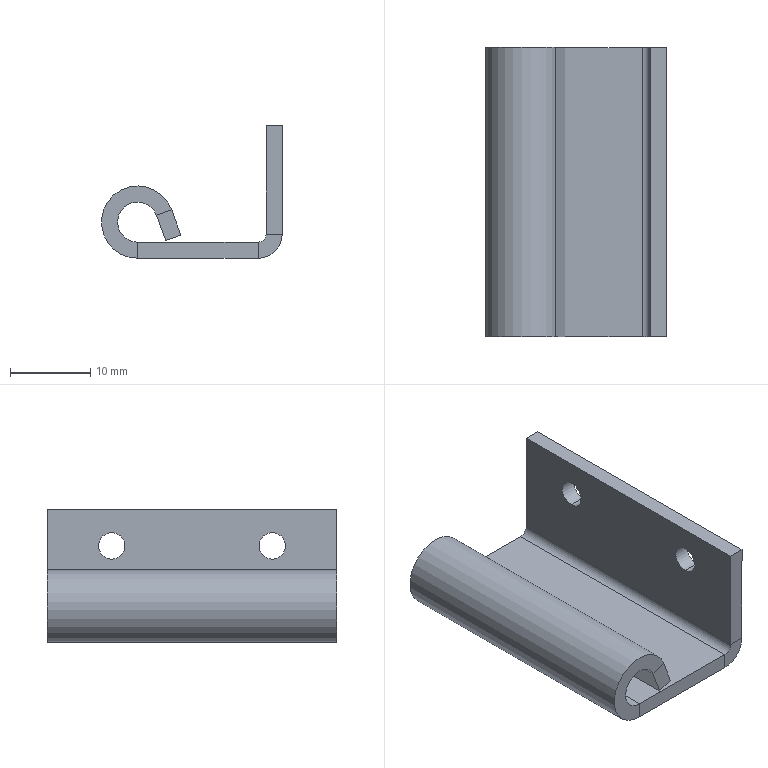Part | SolidWorks | features EdgeFlange 1, FlatPattern 1, Hem 1, HoleWzd 1, SMBaseFlange 1, SheetMetal 1 | 1 solid | 26 faces | box 22.5 x 36 x 16.5 mm | volume 3586 mm3 | plane 18 | cylinder 8 | commonest cylinder face diameters 3.3 x4 2 x1 5 x1 6 x1 9 x1
STEP:
#1=CARTESIAN_POINT('',(11.25,10.,8.35));
#2=VERTEX_POINT('',#1);
#3=CARTESIAN_POINT('',(11.25,10.,11.65));
#4=VERTEX_POINT('',#3);
#5=CARTESIAN_POINT('',(11.25,10.,10.));
#6=DIRECTION('',(-1.,0.,0.));
#7=DIRECTION('',(0.,0.,1.));
#8=AXIS2_PLACEMENT_3D('',#5,#6,#7);
#9=CIRCLE('',#8,1.65);
#10=EDGE_CURVE('',#2,#4,#9,.T.);
#11=ORIENTED_EDGE('',*,*,#10,.F.);
#12=CARTESIAN_POINT('',(9.25,10.,8.35));
#13=VERTEX_POINT('',#12);
#14=CARTESIAN_POINT('',(9.25,10.,8.35));
#15=DIRECTION('',(-1.,0.,0.));
#16=VECTOR('',#15,1000.);
#17=LINE('',#14,#16);
#18=EDGE_CURVE('',#2,#13,#17,.T.);
#19=ORIENTED_EDGE('',*,*,#18,.T.);
#20=CARTESIAN_POINT('',(9.25,10.,11.65));
#21=VERTEX_POINT('',#20);
#22=CARTESIAN_POINT('',(9.25,10.,10.));
#23=DIRECTION('',(-1.,0.,0.));
#24=DIRECTION('',(0.,0.,1.));
#25=AXIS2_PLACEMENT_3D('',#22,#23,#24);
#26=CIRCLE('',#25,1.65);
#27=EDGE_CURVE('',#13,#21,#26,.T.);
#28=ORIENTED_EDGE('',*,*,#27,.T.);
#29=CARTESIAN_POINT('',(9.25,10.,11.65));
#30=DIRECTION('',(-1.,0.,0.));
#31=VECTOR('',#30,1000.);
#32=LINE('',#29,#31);
#33=EDGE_CURVE('',#4,#21,#32,.T.);
#34=ORIENTED_EDGE('',*,*,#33,.F.);
#35=EDGE_LOOP('',(#11,#19,#28,#34));
#36=FACE_OUTER_BOUND('',#35,.T.);
#37=CARTESIAN_POINT('',(9.25,10.,10.));
#38=DIRECTION('',(-1.,0.,0.));
#39=DIRECTION('',(0.,0.,1.));
#40=AXIS2_PLACEMENT_3D('',#37,#38,#39);
#41=CYLINDRICAL_SURFACE('',#40,1.65);
#42=ADVANCED_FACE('',(#36),#41,.F.);
#43=CARTESIAN_POINT('',(11.25,-10.,8.35));
#44=VERTEX_POINT('',#43);
#45=CARTESIAN_POINT('',(11.25,-10.,11.65));
#46=VERTEX_POINT('',#45);
#47=CARTESIAN_POINT('',(11.25,-10.,10.));
#48=DIRECTION('',(-1.,0.,0.));
#49=DIRECTION('',(0.,0.,1.));
#50=AXIS2_PLACEMENT_3D('',#47,#48,#49);
#51=CIRCLE('',#50,1.65);
#52=EDGE_CURVE('',#44,#46,#51,.T.);
#53=ORIENTED_EDGE('',*,*,#52,.F.);
#54=CARTESIAN_POINT('',(9.25,-10.,8.35));
#55=VERTEX_POINT('',#54);
#56=CARTESIAN_POINT('',(9.25,-10.,8.35));
#57=DIRECTION('',(-1.,0.,0.));
#58=VECTOR('',#57,1000.);
#59=LINE('',#56,#58);
#60=EDGE_CURVE('',#44,#55,#59,.T.);
#61=ORIENTED_EDGE('',*,*,#60,.T.);
#62=CARTESIAN_POINT('',(9.25,-10.,11.65));
#63=VERTEX_POINT('',#62);
#64=CARTESIAN_POINT('',(9.25,-10.,10.));
#65=DIRECTION('',(-1.,0.,0.));
#66=DIRECTION('',(0.,0.,1.));
#67=AXIS2_PLACEMENT_3D('',#64,#65,#66);
#68=CIRCLE('',#67,1.65);
#69=EDGE_CURVE('',#55,#63,#68,.T.);
#70=ORIENTED_EDGE('',*,*,#69,.T.);
#71=CARTESIAN_POINT('',(9.25,-10.,11.65));
#72=DIRECTION('',(-1.,0.,0.));
#73=VECTOR('',#72,1000.);
#74=LINE('',#71,#73);
#75=EDGE_CURVE('',#46,#63,#74,.T.);
#76=ORIENTED_EDGE('',*,*,#75,.F.);
#77=EDGE_LOOP('',(#53,#61,#70,#76));
#78=FACE_OUTER_BOUND('',#77,.T.);
#79=CARTESIAN_POINT('',(9.25,-10.,10.));
#80=DIRECTION('',(-1.,0.,0.));
#81=DIRECTION('',(0.,0.,1.));
#82=AXIS2_PLACEMENT_3D('',#79,#80,#81);
#83=CYLINDRICAL_SURFACE('',#82,1.65);
#84=ADVANCED_FACE('',(#78),#83,.F.);
#85=CARTESIAN_POINT('',(8.25,18.,0.));
#86=VERTEX_POINT('',#85);
#87=CARTESIAN_POINT('',(-6.75,18.,0.));
#88=VERTEX_POINT('',#87);
#89=CARTESIAN_POINT('',(-11.25,18.,0.));
#90=DIRECTION('',(-1.,0.,0.));
#91=VECTOR('',#90,1000.);
#92=LINE('',#89,#91);
#93=EDGE_CURVE('',#86,#88,#92,.T.);
#94=ORIENTED_EDGE('',*,*,#93,.F.);
#95=CARTESIAN_POINT('',(8.25,18.,-2.));
#96=VERTEX_POINT('',#95);
#97=CARTESIAN_POINT('',(8.25,18.,0.));
#98=DIRECTION('',(0.,0.,-1.));
#99=VECTOR('',#98,1000.);
#100=LINE('',#97,#99);
#101=EDGE_CURVE('',#86,#96,#100,.T.);
#102=ORIENTED_EDGE('',*,*,#101,.T.);
#103=CARTESIAN_POINT('',(-6.75,18.,-2.));
#104=VERTEX_POINT('',#103);
#105=CARTESIAN_POINT('',(-11.25,18.,-2.));
#106=DIRECTION('',(-1.,0.,0.));
#107=VECTOR('',#106,1000.);
#108=LINE('',#105,#107);
#109=EDGE_CURVE('',#96,#104,#108,.T.);
#110=ORIENTED_EDGE('',*,*,#109,.T.);
#111=CARTESIAN_POINT('',(-6.75,18.,0.));
#112=DIRECTION('',(0.,0.,-1.));
#113=VECTOR('',#112,1000.);
#114=LINE('',#111,#113);
#115=EDGE_CURVE('',#88,#104,#114,.T.);
#116=ORIENTED_EDGE('',*,*,#115,.F.);
#117=EDGE_LOOP('',(#94,#102,#110,#116));
#118=FACE_OUTER_BOUND('',#117,.T.);
#119=CARTESIAN_POINT('',(-11.25,18.,-2.));
#120=DIRECTION('',(0.,1.,0.));
#121=DIRECTION('',(0.,0.,1.));
#122=AXIS2_PLACEMENT_3D('',#119,#120,#121);
#123=PLANE('',#122);
#124=ADVANCED_FACE('',(#118),#123,.T.);
#125=ORIENTED_EDGE('',*,*,#109,.F.);
#126=CARTESIAN_POINT('',(8.25,-18.,-2.));
#127=VERTEX_POINT('',#126);
#128=CARTESIAN_POINT('',(8.25,18.,-2.));
#129=DIRECTION('',(0.,-1.,0.));
#130=VECTOR('',#129,1000.);
#131=LINE('',#128,#130);
#132=EDGE_CURVE('',#96,#127,#131,.T.);
#133=ORIENTED_EDGE('',*,*,#132,.T.);
#134=CARTESIAN_POINT('',(-6.75,-18.,-2.));
#135=VERTEX_POINT('',#134);
#136=CARTESIAN_POINT('',(-11.25,-18.,-2.));
#137=DIRECTION('',(1.,0.,0.));
#138=VECTOR('',#137,1000.);
#139=LINE('',#136,#138);
#140=EDGE_CURVE('',#135,#127,#139,.T.);
#141=ORIENTED_EDGE('',*,*,#140,.F.);
#142=CARTESIAN_POINT('',(-6.75,-18.,-2.));
#143=DIRECTION('',(0.,1.,0.));
#144=VECTOR('',#143,1000.);
#145=LINE('',#142,#144);
#146=EDGE_CURVE('',#135,#104,#145,.T.);
#147=ORIENTED_EDGE('',*,*,#146,.T.);
#148=EDGE_LOOP('',(#125,#133,#141,#147));
#149=FACE_OUTER_BOUND('',#148,.T.);
#150=CARTESIAN_POINT('',(0.,0.,-2.));
#151=DIRECTION('',(0.,0.,-1.));
#152=DIRECTION('',(-1.,0.,0.));
#153=AXIS2_PLACEMENT_3D('',#150,#151,#152);
#154=PLANE('',#153);
#155=ADVANCED_FACE('',(#149),#154,.T.);
#156=CARTESIAN_POINT('',(8.25,-18.,0.));
#157=VERTEX_POINT('',#156);
#158=CARTESIAN_POINT('',(8.25,18.,0.));
#159=DIRECTION('',(0.,-1.,0.));
#160=VECTOR('',#159,1000.);
#161=LINE('',#158,#160);
#162=EDGE_CURVE('',#86,#157,#161,.T.);
#163=ORIENTED_EDGE('',*,*,#162,.F.);
#164=ORIENTED_EDGE('',*,*,#93,.T.);
#165=CARTESIAN_POINT('',(-6.75,-18.,0.));
#166=VERTEX_POINT('',#165);
#167=CARTESIAN_POINT('',(-6.75,-18.,0.));
#168=DIRECTION('',(0.,1.,0.));
#169=VECTOR('',#168,1000.);
#170=LINE('',#167,#169);
#171=EDGE_CURVE('',#166,#88,#170,.T.);
#172=ORIENTED_EDGE('',*,*,#171,.F.);
#173=CARTESIAN_POINT('',(-11.25,-18.,0.));
#174=DIRECTION('',(1.,0.,0.));
#175=VECTOR('',#174,1000.);
#176=LINE('',#173,#175);
#177=EDGE_CURVE('',#166,#157,#176,.T.);
#178=ORIENTED_EDGE('',*,*,#177,.T.);
#179=EDGE_LOOP('',(#163,#164,#172,#178));
#180=FACE_OUTER_BOUND('',#179,.T.);
#181=CARTESIAN_POINT('',(0.,0.,0.));
#182=DIRECTION('',(0.,0.,-1.));
#183=DIRECTION('',(-1.,0.,0.));
#184=AXIS2_PLACEMENT_3D('',#181,#182,#183);
#185=PLANE('',#184);
#186=ADVANCED_FACE('',(#180),#185,.F.);
#187=CARTESIAN_POINT('',(8.25,-18.,0.));
#188=DIRECTION('',(0.,0.,-1.));
#189=VECTOR('',#188,1000.);
#190=LINE('',#187,#189);
#191=EDGE_CURVE('',#157,#127,#190,.T.);
#192=ORIENTED_EDGE('',*,*,#191,.F.);
#193=ORIENTED_EDGE('',*,*,#177,.F.);
#194=CARTESIAN_POINT('',(-6.75,-18.,0.));
#195=DIRECTION('',(0.,0.,-1.));
#196=VECTOR('',#195,1000.);
#197=LINE('',#194,#196);
#198=EDGE_CURVE('',#166,#135,#197,.T.);
#199=ORIENTED_EDGE('',*,*,#198,.T.);
#200=ORIENTED_EDGE('',*,*,#140,.T.);
#201=EDGE_LOOP('',(#192,#193,#199,#200));
#202=FACE_OUTER_BOUND('',#201,.T.);
#203=CARTESIAN_POINT('',(-11.25,-18.,-2.));
#204=DIRECTION('',(0.,-1.,0.));
#205=DIRECTION('',(0.,0.,-1.));
#206=AXIS2_PLACEMENT_3D('',#203,#204,#205);
#207=PLANE('',#206);
#208=ADVANCED_FACE('',(#202),#207,.T.);
#209=CARTESIAN_POINT('',(-4.401,-18.,3.355));
#210=VERTEX_POINT('',#209);
#211=CARTESIAN_POINT('',(-2.521,-18.,4.039));
#212=VERTEX_POINT('',#211);
#213=CARTESIAN_POINT('',(-2.521,-18.,4.039));
#214=DIRECTION('',(0.9397,0.,0.342));
#215=VECTOR('',#214,1000.);
#216=LINE('',#213,#215);
#217=EDGE_CURVE('',#210,#212,#216,.T.);
#218=ORIENTED_EDGE('',*,*,#217,.F.);
#219=CARTESIAN_POINT('',(-3.248,-18.,0.1879));
#220=VERTEX_POINT('',#219);
#221=CARTESIAN_POINT('',(-3.824,-18.,1.771));
#222=DIRECTION('',(-0.342,0.,0.9397));
#223=VECTOR('',#222,1000.);
#224=LINE('',#221,#223);
#225=EDGE_CURVE('',#220,#210,#224,.T.);
#226=ORIENTED_EDGE('',*,*,#225,.F.);
#227=CARTESIAN_POINT('',(-1.369,-18.,0.872));
#228=VERTEX_POINT('',#227);
#229=CARTESIAN_POINT('',(-1.369,-18.,0.872));
#230=DIRECTION('',(0.9397,0.,0.342));
#231=VECTOR('',#230,1000.);
#232=LINE('',#229,#231);
#233=EDGE_CURVE('',#220,#228,#232,.T.);
#234=ORIENTED_EDGE('',*,*,#233,.T.);
#235=CARTESIAN_POINT('',(-1.945,-18.,2.456));
#236=DIRECTION('',(-0.342,0.,0.9397));
#237=VECTOR('',#236,1000.);
#238=LINE('',#235,#237);
#239=EDGE_CURVE('',#228,#212,#238,.T.);
#240=ORIENTED_EDGE('',*,*,#239,.T.);
#241=EDGE_LOOP('',(#218,#226,#234,#240));
#242=FACE_OUTER_BOUND('',#241,.T.);
#243=CARTESIAN_POINT('',(-1.945,-18.,2.456));
#244=DIRECTION('',(0.,1.,0.));
#245=DIRECTION('',(-0.342,0.,0.9397));
#246=AXIS2_PLACEMENT_3D('',#243,#244,#245);
#247=PLANE('',#246);
#248=ADVANCED_FACE('',(#242),#247,.F.);
#249=ORIENTED_EDGE('',*,*,#233,.F.);
#250=CARTESIAN_POINT('',(-3.248,18.,0.1879));
#251=VERTEX_POINT('',#250);
#252=CARTESIAN_POINT('',(-3.248,0.,0.1879));
#253=DIRECTION('',(0.,-1.,0.));
#254=VECTOR('',#253,1000.);
#255=LINE('',#252,#254);
#256=EDGE_CURVE('',#251,#220,#255,.T.);
#257=ORIENTED_EDGE('',*,*,#256,.F.);
#258=CARTESIAN_POINT('',(-1.369,18.,0.872));
#259=VERTEX_POINT('',#258);
#260=CARTESIAN_POINT('',(-1.369,18.,0.872));
#261=DIRECTION('',(0.9397,0.,0.342));
#262=VECTOR('',#261,1000.);
#263=LINE('',#260,#262);
#264=EDGE_CURVE('',#251,#259,#263,.T.);
#265=ORIENTED_EDGE('',*,*,#264,.T.);
#266=CARTESIAN_POINT('',(-1.369,0.,0.872));
#267=DIRECTION('',(0.,-1.,0.));
#268=VECTOR('',#267,1000.);
#269=LINE('',#266,#268);
#270=EDGE_CURVE('',#259,#228,#269,.T.);
#271=ORIENTED_EDGE('',*,*,#270,.T.);
#272=EDGE_LOOP('',(#249,#257,#265,#271));
#273=FACE_OUTER_BOUND('',#272,.T.);
#274=CARTESIAN_POINT('',(-1.369,0.,0.872));
#275=DIRECTION('',(-0.342,0.,0.9397));
#276=DIRECTION('',(0.,-1.,0.));
#277=AXIS2_PLACEMENT_3D('',#274,#275,#276);
#278=PLANE('',#277);
#279=ADVANCED_FACE('',(#273),#278,.F.);
#280=CARTESIAN_POINT('',(-4.401,18.,3.355));
#281=VERTEX_POINT('',#280);
#282=CARTESIAN_POINT('',(-3.824,18.,1.771));
#283=DIRECTION('',(0.342,0.,-0.9397));
#284=VECTOR('',#283,1000.);
#285=LINE('',#282,#284);
#286=EDGE_CURVE('',#281,#251,#285,.T.);
#287=ORIENTED_EDGE('',*,*,#286,.F.);
#288=CARTESIAN_POINT('',(-2.521,18.,4.039));
#289=VERTEX_POINT('',#288);
#290=CARTESIAN_POINT('',(-2.521,18.,4.039));
#291=DIRECTION('',(0.9397,0.,0.342));
#292=VECTOR('',#291,1000.);
#293=LINE('',#290,#292);
#294=EDGE_CURVE('',#281,#289,#293,.T.);
#295=ORIENTED_EDGE('',*,*,#294,.T.);
#296=CARTESIAN_POINT('',(-1.945,18.,2.456));
#297=DIRECTION('',(0.342,0.,-0.9397));
#298=VECTOR('',#297,1000.);
#299=LINE('',#296,#298);
#300=EDGE_CURVE('',#289,#259,#299,.T.);
#301=ORIENTED_EDGE('',*,*,#300,.T.);
#302=ORIENTED_EDGE('',*,*,#264,.F.);
#303=EDGE_LOOP('',(#287,#295,#301,#302));
#304=FACE_OUTER_BOUND('',#303,.T.);
#305=CARTESIAN_POINT('',(-1.945,18.,2.456));
#306=DIRECTION('',(0.,-1.,0.));
#307=DIRECTION('',(0.342,0.,-0.9397));
#308=AXIS2_PLACEMENT_3D('',#305,#306,#307);
#309=PLANE('',#308);
#310=ADVANCED_FACE('',(#304),#309,.F.);
#311=ORIENTED_EDGE('',*,*,#270,.F.);
#312=ORIENTED_EDGE('',*,*,#300,.F.);
#313=CARTESIAN_POINT('',(-2.521,0.,4.039));
#314=DIRECTION('',(0.,1.,0.));
#315=VECTOR('',#314,1000.);
#316=LINE('',#313,#315);
#317=EDGE_CURVE('',#212,#289,#316,.T.);
#318=ORIENTED_EDGE('',*,*,#317,.F.);
#319=ORIENTED_EDGE('',*,*,#239,.F.);
#320=EDGE_LOOP('',(#311,#312,#318,#319));
#321=FACE_OUTER_BOUND('',#320,.T.);
#322=CARTESIAN_POINT('',(-1.945,0.,2.456));
#323=DIRECTION('',(0.9397,0.,0.342));
#324=DIRECTION('',(0.342,0.,-0.9397));
#325=AXIS2_PLACEMENT_3D('',#322,#323,#324);
#326=PLANE('',#325);
#327=ADVANCED_FACE('',(#321),#326,.T.);
#328=ORIENTED_EDGE('',*,*,#256,.T.);
#329=ORIENTED_EDGE('',*,*,#225,.T.);
#330=CARTESIAN_POINT('',(-4.401,0.,3.355));
#331=DIRECTION('',(0.,1.,0.));
#332=VECTOR('',#331,1000.);
#333=LINE('',#330,#332);
#334=EDGE_CURVE('',#210,#281,#333,.T.);
#335=ORIENTED_EDGE('',*,*,#334,.T.);
#336=ORIENTED_EDGE('',*,*,#286,.T.);
#337=EDGE_LOOP('',(#328,#329,#335,#336));
#338=FACE_OUTER_BOUND('',#337,.T.);
#339=CARTESIAN_POINT('',(-3.824,0.,1.771));
#340=DIRECTION('',(0.9397,0.,0.342));
#341=DIRECTION('',(0.342,0.,-0.9397));
#342=AXIS2_PLACEMENT_3D('',#339,#340,#341);
#343=PLANE('',#342);
#344=ADVANCED_FACE('',(#338),#343,.F.);
#345=ORIENTED_EDGE('',*,*,#294,.F.);
#346=CARTESIAN_POINT('',(-6.75,18.,2.5));
#347=DIRECTION('',(0.,1.,0.));
#348=DIRECTION('',(0.,0.,-1.));
#349=AXIS2_PLACEMENT_3D('',#346,#347,#348);
#350=CIRCLE('',#349,2.5);
#351=EDGE_CURVE('',#88,#281,#350,.T.);
#352=ORIENTED_EDGE('',*,*,#351,.F.);
#353=ORIENTED_EDGE('',*,*,#115,.T.);
#354=CARTESIAN_POINT('',(-6.75,18.,2.5));
#355=DIRECTION('',(0.,1.,0.));
#356=DIRECTION('',(0.,0.,-1.));
#357=AXIS2_PLACEMENT_3D('',#354,#355,#356);
#358=CIRCLE('',#357,4.5);
#359=EDGE_CURVE('',#104,#289,#358,.T.);
#360=ORIENTED_EDGE('',*,*,#359,.T.);
#361=EDGE_LOOP('',(#345,#352,#353,#360));
#362=FACE_OUTER_BOUND('',#361,.T.);
#363=CARTESIAN_POINT('',(-6.75,18.,2.5));
#364=DIRECTION('',(0.,1.,0.));
#365=DIRECTION('',(0.,0.,1.));
#366=AXIS2_PLACEMENT_3D('',#363,#364,#365);
#367=PLANE('',#366);
#368=ADVANCED_FACE('',(#362),#367,.T.);
#369=CARTESIAN_POINT('',(-6.75,-18.,2.5));
#370=DIRECTION('',(0.,-1.,0.));
#371=DIRECTION('',(0.,0.,-1.));
#372=AXIS2_PLACEMENT_3D('',#369,#370,#371);
#373=CIRCLE('',#372,2.5);
#374=EDGE_CURVE('',#210,#166,#373,.T.);
#375=ORIENTED_EDGE('',*,*,#374,.F.);
#376=ORIENTED_EDGE('',*,*,#217,.T.);
#377=CARTESIAN_POINT('',(-6.75,-18.,2.5));
#378=DIRECTION('',(0.,-1.,0.));
#379=DIRECTION('',(0.,0.,-1.));
#380=AXIS2_PLACEMENT_3D('',#377,#378,#379);
#381=CIRCLE('',#380,4.5);
#382=EDGE_CURVE('',#212,#135,#381,.T.);
#383=ORIENTED_EDGE('',*,*,#382,.T.);
#384=ORIENTED_EDGE('',*,*,#198,.F.);
#385=EDGE_LOOP('',(#375,#376,#383,#384));
#386=FACE_OUTER_BOUND('',#385,.T.);
#387=CARTESIAN_POINT('',(-6.75,-18.,2.5));
#388=DIRECTION('',(0.,1.,0.));
#389=DIRECTION('',(0.,0.,1.));
#390=AXIS2_PLACEMENT_3D('',#387,#388,#389);
#391=PLANE('',#390);
#392=ADVANCED_FACE('',(#386),#391,.F.);
#393=ORIENTED_EDGE('',*,*,#146,.F.);
#394=ORIENTED_EDGE('',*,*,#382,.F.);
#395=ORIENTED_EDGE('',*,*,#317,.T.);
#396=ORIENTED_EDGE('',*,*,#359,.F.);
#397=EDGE_LOOP('',(#393,#394,#395,#396));
#398=FACE_OUTER_BOUND('',#397,.T.);
#399=CARTESIAN_POINT('',(-6.75,-18.,2.5));
#400=DIRECTION('',(0.,-1.,0.));
#401=DIRECTION('',(0.9397,0.,0.342));
#402=AXIS2_PLACEMENT_3D('',#399,#400,#401);
#403=CYLINDRICAL_SURFACE('',#402,4.5);
#404=ADVANCED_FACE('',(#398),#403,.T.);
#405=ORIENTED_EDGE('',*,*,#171,.T.);
#406=ORIENTED_EDGE('',*,*,#351,.T.);
#407=ORIENTED_EDGE('',*,*,#334,.F.);
#408=ORIENTED_EDGE('',*,*,#374,.T.);
#409=EDGE_LOOP('',(#405,#406,#407,#408));
#410=FACE_OUTER_BOUND('',#409,.T.);
#411=CARTESIAN_POINT('',(-6.75,-18.,2.5));
#412=DIRECTION('',(0.,-1.,0.));
#413=DIRECTION('',(0.9397,0.,0.342));
#414=AXIS2_PLACEMENT_3D('',#411,#412,#413);
#415=CYLINDRICAL_SURFACE('',#414,2.5);
#416=ADVANCED_FACE('',(#410),#415,.F.);
#417=CARTESIAN_POINT('',(9.25,-18.,1.));
#418=VERTEX_POINT('',#417);
#419=CARTESIAN_POINT('',(11.25,-18.,1.));
#420=VERTEX_POINT('',#419);
#421=CARTESIAN_POINT('',(11.25,-18.,1.));
#422=DIRECTION('',(1.,0.,0.));
#423=VECTOR('',#422,1000.);
#424=LINE('',#421,#423);
#425=EDGE_CURVE('',#418,#420,#424,.T.);
#426=ORIENTED_EDGE('',*,*,#425,.F.);
#427=CARTESIAN_POINT('',(8.25,-18.,1.));
#428=DIRECTION('',(0.,-1.,0.));
#429=DIRECTION('',(0.,0.,1.));
#430=AXIS2_PLACEMENT_3D('',#427,#428,#429);
#431=CIRCLE('',#430,1.);
#432=EDGE_CURVE('',#157,#418,#431,.T.);
#433=ORIENTED_EDGE('',*,*,#432,.F.);
#434=ORIENTED_EDGE('',*,*,#191,.T.);
#435=CARTESIAN_POINT('',(8.25,-18.,1.));
#436=DIRECTION('',(0.,-1.,0.));
#437=DIRECTION('',(0.,0.,1.));
#438=AXIS2_PLACEMENT_3D('',#435,#436,#437);
#439=CIRCLE('',#438,3.);
#440=EDGE_CURVE('',#127,#420,#439,.T.);
#441=ORIENTED_EDGE('',*,*,#440,.T.);
#442=EDGE_LOOP('',(#426,#433,#434,#441));
#443=FACE_OUTER_BOUND('',#442,.T.);
#444=CARTESIAN_POINT('',(8.25,-18.,1.));
#445=DIRECTION('',(0.,-1.,0.));
#446=DIRECTION('',(0.,0.,-1.));
#447=AXIS2_PLACEMENT_3D('',#444,#445,#446);
#448=PLANE('',#447);
#449=ADVANCED_FACE('',(#443),#448,.T.);
#450=CARTESIAN_POINT('',(9.25,18.,1.));
#451=VERTEX_POINT('',#450);
#452=CARTESIAN_POINT('',(8.25,18.,1.));
#453=DIRECTION('',(0.,1.,0.));
#454=DIRECTION('',(0.,0.,1.));
#455=AXIS2_PLACEMENT_3D('',#452,#453,#454);
#456=CIRCLE('',#455,1.);
#457=EDGE_CURVE('',#451,#86,#456,.T.);
#458=ORIENTED_EDGE('',*,*,#457,.F.);
#459=CARTESIAN_POINT('',(11.25,18.,1.));
#460=VERTEX_POINT('',#459);
#461=CARTESIAN_POINT('',(9.25,18.,1.));
#462=DIRECTION('',(1.,0.,0.));
#463=VECTOR('',#462,1000.);
#464=LINE('',#461,#463);
#465=EDGE_CURVE('',#451,#460,#464,.T.);
#466=ORIENTED_EDGE('',*,*,#465,.T.);
#467=CARTESIAN_POINT('',(8.25,18.,1.));
#468=DIRECTION('',(0.,1.,0.));
#469=DIRECTION('',(0.,0.,1.));
#470=AXIS2_PLACEMENT_3D('',#467,#468,#469);
#471=CIRCLE('',#470,3.);
#472=EDGE_CURVE('',#460,#96,#471,.T.);
#473=ORIENTED_EDGE('',*,*,#472,.T.);
#474=ORIENTED_EDGE('',*,*,#101,.F.);
#475=EDGE_LOOP('',(#458,#466,#473,#474));
#476=FACE_OUTER_BOUND('',#475,.T.);
#477=CARTESIAN_POINT('',(8.25,18.,1.));
#478=DIRECTION('',(0.,-1.,0.));
#479=DIRECTION('',(0.,0.,-1.));
#480=AXIS2_PLACEMENT_3D('',#477,#478,#479);
#481=PLANE('',#480);
#482=ADVANCED_FACE('',(#476),#481,.F.);
#483=ORIENTED_EDGE('',*,*,#132,.F.);
#484=ORIENTED_EDGE('',*,*,#472,.F.);
#485=CARTESIAN_POINT('',(11.25,-18.,1.));
#486=DIRECTION('',(0.,-1.,0.));
#487=VECTOR('',#486,1000.);
#488=LINE('',#485,#487);
#489=EDGE_CURVE('',#460,#420,#488,.T.);
#490=ORIENTED_EDGE('',*,*,#489,.T.);
#491=ORIENTED_EDGE('',*,*,#440,.F.);
#492=EDGE_LOOP('',(#483,#484,#490,#491));
#493=FACE_OUTER_BOUND('',#492,.T.);
#494=CARTESIAN_POINT('',(8.25,18.,1.));
#495=DIRECTION('',(0.,1.,0.));
#496=DIRECTION('',(1.,0.,0.));
#497=AXIS2_PLACEMENT_3D('',#494,#495,#496);
#498=CYLINDRICAL_SURFACE('',#497,3.);
#499=ADVANCED_FACE('',(#493),#498,.T.);
#500=ORIENTED_EDGE('',*,*,#162,.T.);
#501=ORIENTED_EDGE('',*,*,#432,.T.);
#502=CARTESIAN_POINT('',(9.25,-18.,1.));
#503=DIRECTION('',(0.,1.,0.));
#504=VECTOR('',#503,1000.);
#505=LINE('',#502,#504);
#506=EDGE_CURVE('',#418,#451,#505,.T.);
#507=ORIENTED_EDGE('',*,*,#506,.T.);
#508=ORIENTED_EDGE('',*,*,#457,.T.);
#509=EDGE_LOOP('',(#500,#501,#507,#508));
#510=FACE_OUTER_BOUND('',#509,.T.);
#511=CARTESIAN_POINT('',(8.25,18.,1.));
#512=DIRECTION('',(0.,1.,0.));
#513=DIRECTION('',(1.,0.,0.));
#514=AXIS2_PLACEMENT_3D('',#511,#512,#513);
#515=CYLINDRICAL_SURFACE('',#514,1.);
#516=ADVANCED_FACE('',(#510),#515,.F.);
#517=ORIENTED_EDGE('',*,*,#425,.T.);
#518=CARTESIAN_POINT('',(11.25,-18.,14.5));
#519=VERTEX_POINT('',#518);
#520=CARTESIAN_POINT('',(11.25,-18.,0.));
#521=DIRECTION('',(0.,0.,-1.));
#522=VECTOR('',#521,1000.);
#523=LINE('',#520,#522);
#524=EDGE_CURVE('',#519,#420,#523,.T.);
#525=ORIENTED_EDGE('',*,*,#524,.F.);
#526=CARTESIAN_POINT('',(9.25,-18.,14.5));
#527=VERTEX_POINT('',#526);
#528=CARTESIAN_POINT('',(11.25,-18.,14.5));
#529=DIRECTION('',(-1.,0.,0.));
#530=VECTOR('',#529,1000.);
#531=LINE('',#528,#530);
#532=EDGE_CURVE('',#519,#527,#531,.T.);
#533=ORIENTED_EDGE('',*,*,#532,.T.);
#534=CARTESIAN_POINT('',(9.25,-18.,0.));
#535=DIRECTION('',(0.,0.,-1.));
#536=VECTOR('',#535,1000.);
#537=LINE('',#534,#536);
#538=EDGE_CURVE('',#527,#418,#537,.T.);
#539=ORIENTED_EDGE('',*,*,#538,.T.);
#540=EDGE_LOOP('',(#517,#525,#533,#539));
#541=FACE_OUTER_BOUND('',#540,.T.);
#542=CARTESIAN_POINT('',(11.25,-18.,0.));
#543=DIRECTION('',(0.,1.,0.));
#544=DIRECTION('',(0.,0.,1.));
#545=AXIS2_PLACEMENT_3D('',#542,#543,#544);
#546=PLANE('',#545);
#547=ADVANCED_FACE('',(#541),#546,.F.);
#548=ORIENTED_EDGE('',*,*,#465,.F.);
#549=CARTESIAN_POINT('',(9.25,18.,14.5));
#550=VERTEX_POINT('',#549);
#551=CARTESIAN_POINT('',(9.25,18.,14.5));
#552=DIRECTION('',(0.,0.,1.));
#553=VECTOR('',#552,1000.);
#554=LINE('',#551,#553);
#555=EDGE_CURVE('',#451,#550,#554,.T.);
#556=ORIENTED_EDGE('',*,*,#555,.T.);
#557=CARTESIAN_POINT('',(11.25,18.,14.5));
#558=VERTEX_POINT('',#557);
#559=CARTESIAN_POINT('',(11.25,18.,14.5));
#560=DIRECTION('',(-1.,0.,0.));
#561=VECTOR('',#560,1000.);
#562=LINE('',#559,#561);
#563=EDGE_CURVE('',#558,#550,#562,.T.);
#564=ORIENTED_EDGE('',*,*,#563,.F.);
#565=CARTESIAN_POINT('',(11.25,18.,0.));
#566=DIRECTION('',(0.,0.,1.));
#567=VECTOR('',#566,1000.);
#568=LINE('',#565,#567);
#569=EDGE_CURVE('',#460,#558,#568,.T.);
#570=ORIENTED_EDGE('',*,*,#569,.F.);
#571=EDGE_LOOP('',(#548,#556,#564,#570));
#572=FACE_OUTER_BOUND('',#571,.T.);
#573=CARTESIAN_POINT('',(11.25,18.,14.5));
#574=DIRECTION('',(0.,-1.,0.));
#575=DIRECTION('',(0.,0.,-1.));
#576=AXIS2_PLACEMENT_3D('',#573,#574,#575);
#577=PLANE('',#576);
#578=ADVANCED_FACE('',(#572),#577,.F.);
#579=CARTESIAN_POINT('',(11.25,10.,10.));
#580=DIRECTION('',(-1.,0.,0.));
#581=DIRECTION('',(0.,0.,1.));
#582=AXIS2_PLACEMENT_3D('',#579,#580,#581);
#583=CIRCLE('',#582,1.65);
#584=EDGE_CURVE('',#4,#2,#583,.T.);
#585=ORIENTED_EDGE('',*,*,#584,.T.);
#586=ORIENTED_EDGE('',*,*,#10,.T.);
#587=EDGE_LOOP('',(#585,#586));
#588=FACE_BOUND('',#587,.T.);
#589=CARTESIAN_POINT('',(11.25,-10.,10.));
#590=DIRECTION('',(-1.,0.,0.));
#591=DIRECTION('',(0.,0.,1.));
#592=AXIS2_PLACEMENT_3D('',#589,#590,#591);
#593=CIRCLE('',#592,1.65);
#594=EDGE_CURVE('',#46,#44,#593,.T.);
#595=ORIENTED_EDGE('',*,*,#594,.T.);
#596=ORIENTED_EDGE('',*,*,#52,.T.);
#597=EDGE_LOOP('',(#595,#596));
#598=FACE_BOUND('',#597,.T.);
#599=ORIENTED_EDGE('',*,*,#489,.F.);
#600=ORIENTED_EDGE('',*,*,#569,.T.);
#601=CARTESIAN_POINT('',(11.25,0.,14.5));
#602=DIRECTION('',(0.,-1.,0.));
#603=VECTOR('',#602,1000.);
#604=LINE('',#601,#603);
#605=EDGE_CURVE('',#558,#519,#604,.T.);
#606=ORIENTED_EDGE('',*,*,#605,.T.);
#607=ORIENTED_EDGE('',*,*,#524,.T.);
#608=EDGE_LOOP('',(#599,#600,#606,#607));
#609=FACE_OUTER_BOUND('',#608,.T.);
#610=CARTESIAN_POINT('',(11.25,0.,0.));
#611=DIRECTION('',(-1.,0.,0.));
#612=DIRECTION('',(0.,0.,1.));
#613=AXIS2_PLACEMENT_3D('',#610,#611,#612);
#614=PLANE('',#613);
#615=ADVANCED_FACE('',(#588,#598,#609),#614,.F.);
#616=CARTESIAN_POINT('',(9.25,10.,10.));
#617=DIRECTION('',(-1.,0.,0.));
#618=DIRECTION('',(0.,0.,1.));
#619=AXIS2_PLACEMENT_3D('',#616,#617,#618);
#620=CIRCLE('',#619,1.65);
#621=EDGE_CURVE('',#21,#13,#620,.T.);
#622=ORIENTED_EDGE('',*,*,#621,.F.);
#623=ORIENTED_EDGE('',*,*,#27,.F.);
#624=EDGE_LOOP('',(#622,#623));
#625=FACE_BOUND('',#624,.T.);
#626=CARTESIAN_POINT('',(9.25,-10.,10.));
#627=DIRECTION('',(-1.,0.,0.));
#628=DIRECTION('',(0.,0.,1.));
#629=AXIS2_PLACEMENT_3D('',#626,#627,#628);
#630=CIRCLE('',#629,1.65);
#631=EDGE_CURVE('',#63,#55,#630,.T.);
#632=ORIENTED_EDGE('',*,*,#631,.F.);
#633=ORIENTED_EDGE('',*,*,#69,.F.);
#634=EDGE_LOOP('',(#632,#633));
#635=FACE_BOUND('',#634,.T.);
#636=ORIENTED_EDGE('',*,*,#555,.F.);
#637=ORIENTED_EDGE('',*,*,#506,.F.);
#638=ORIENTED_EDGE('',*,*,#538,.F.);
#639=CARTESIAN_POINT('',(9.25,-18.,14.5));
#640=DIRECTION('',(0.,-1.,0.));
#641=VECTOR('',#640,1000.);
#642=LINE('',#639,#641);
#643=EDGE_CURVE('',#550,#527,#642,.T.);
#644=ORIENTED_EDGE('',*,*,#643,.F.);
#645=EDGE_LOOP('',(#636,#637,#638,#644));
#646=FACE_OUTER_BOUND('',#645,.T.);
#647=CARTESIAN_POINT('',(9.25,0.,0.));
#648=DIRECTION('',(-1.,0.,0.));
#649=DIRECTION('',(0.,0.,1.));
#650=AXIS2_PLACEMENT_3D('',#647,#648,#649);
#651=PLANE('',#650);
#652=ADVANCED_FACE('',(#625,#635,#646),#651,.T.);
#653=ORIENTED_EDGE('',*,*,#643,.T.);
#654=ORIENTED_EDGE('',*,*,#532,.F.);
#655=ORIENTED_EDGE('',*,*,#605,.F.);
#656=ORIENTED_EDGE('',*,*,#563,.T.);
#657=EDGE_LOOP('',(#653,#654,#655,#656));
#658=FACE_OUTER_BOUND('',#657,.T.);
#659=CARTESIAN_POINT('',(11.25,-18.,14.5));
#660=DIRECTION('',(0.,0.,-1.));
#661=DIRECTION('',(-1.,0.,0.));
#662=AXIS2_PLACEMENT_3D('',#659,#660,#661);
#663=PLANE('',#662);
#664=ADVANCED_FACE('',(#658),#663,.F.);
#665=ORIENTED_EDGE('',*,*,#60,.F.);
#666=ORIENTED_EDGE('',*,*,#594,.F.);
#667=ORIENTED_EDGE('',*,*,#75,.T.);
#668=ORIENTED_EDGE('',*,*,#631,.T.);
#669=EDGE_LOOP('',(#665,#666,#667,#668));
#670=FACE_OUTER_BOUND('',#669,.T.);
#671=CARTESIAN_POINT('',(9.25,-10.,10.));
#672=DIRECTION('',(-1.,0.,0.));
#673=DIRECTION('',(0.,0.,1.));
#674=AXIS2_PLACEMENT_3D('',#671,#672,#673);
#675=CYLINDRICAL_SURFACE('',#674,1.65);
#676=ADVANCED_FACE('',(#670),#675,.F.);
#677=ORIENTED_EDGE('',*,*,#18,.F.);
#678=ORIENTED_EDGE('',*,*,#584,.F.);
#679=ORIENTED_EDGE('',*,*,#33,.T.);
#680=ORIENTED_EDGE('',*,*,#621,.T.);
#681=EDGE_LOOP('',(#677,#678,#679,#680));
#682=FACE_OUTER_BOUND('',#681,.T.);
#683=CARTESIAN_POINT('',(9.25,10.,10.));
#684=DIRECTION('',(-1.,0.,0.));
#685=DIRECTION('',(0.,0.,1.));
#686=AXIS2_PLACEMENT_3D('',#683,#684,#685);
#687=CYLINDRICAL_SURFACE('',#686,1.65);
#688=ADVANCED_FACE('',(#682),#687,.F.);
#689=CLOSED_SHELL('',(#42,#84,#124,#155,#186,#208,#248,#279,#310,#327,#344,#368,#392,#404,#416,#449,#482,#499,#516,#547,#578,#615,#652,#664,#676,#688));
#690=MANIFOLD_SOLID_BREP('',#689);
#691=CARTESIAN_POINT('',(0.,0.,0.));
#692=DIRECTION('',(0.,0.,1.));
#693=DIRECTION('',(1.,0.,0.));
#694=AXIS2_PLACEMENT_3D('',#691,#692,#693);
#695=(LENGTH_UNIT()NAMED_UNIT(*)SI_UNIT(.MILLI.,.METRE.));
#696=UNCERTAINTY_MEASURE_WITH_UNIT(LENGTH_MEASURE(0.00001),#695,'','');
#697=(NAMED_UNIT(*)PLANE_ANGLE_UNIT()SI_UNIT($,.RADIAN.));
#698=(NAMED_UNIT(*)SI_UNIT($,.STERADIAN.)SOLID_ANGLE_UNIT());
#699=(GEOMETRIC_REPRESENTATION_CONTEXT(3)GLOBAL_UNCERTAINTY_ASSIGNED_CONTEXT((#696))GLOBAL_UNIT_ASSIGNED_CONTEXT((#695,#697,#698))REPRESENTATION_CONTEXT('',''));
#700=ADVANCED_BREP_SHAPE_REPRESENTATION('',(#690,#694),#699);